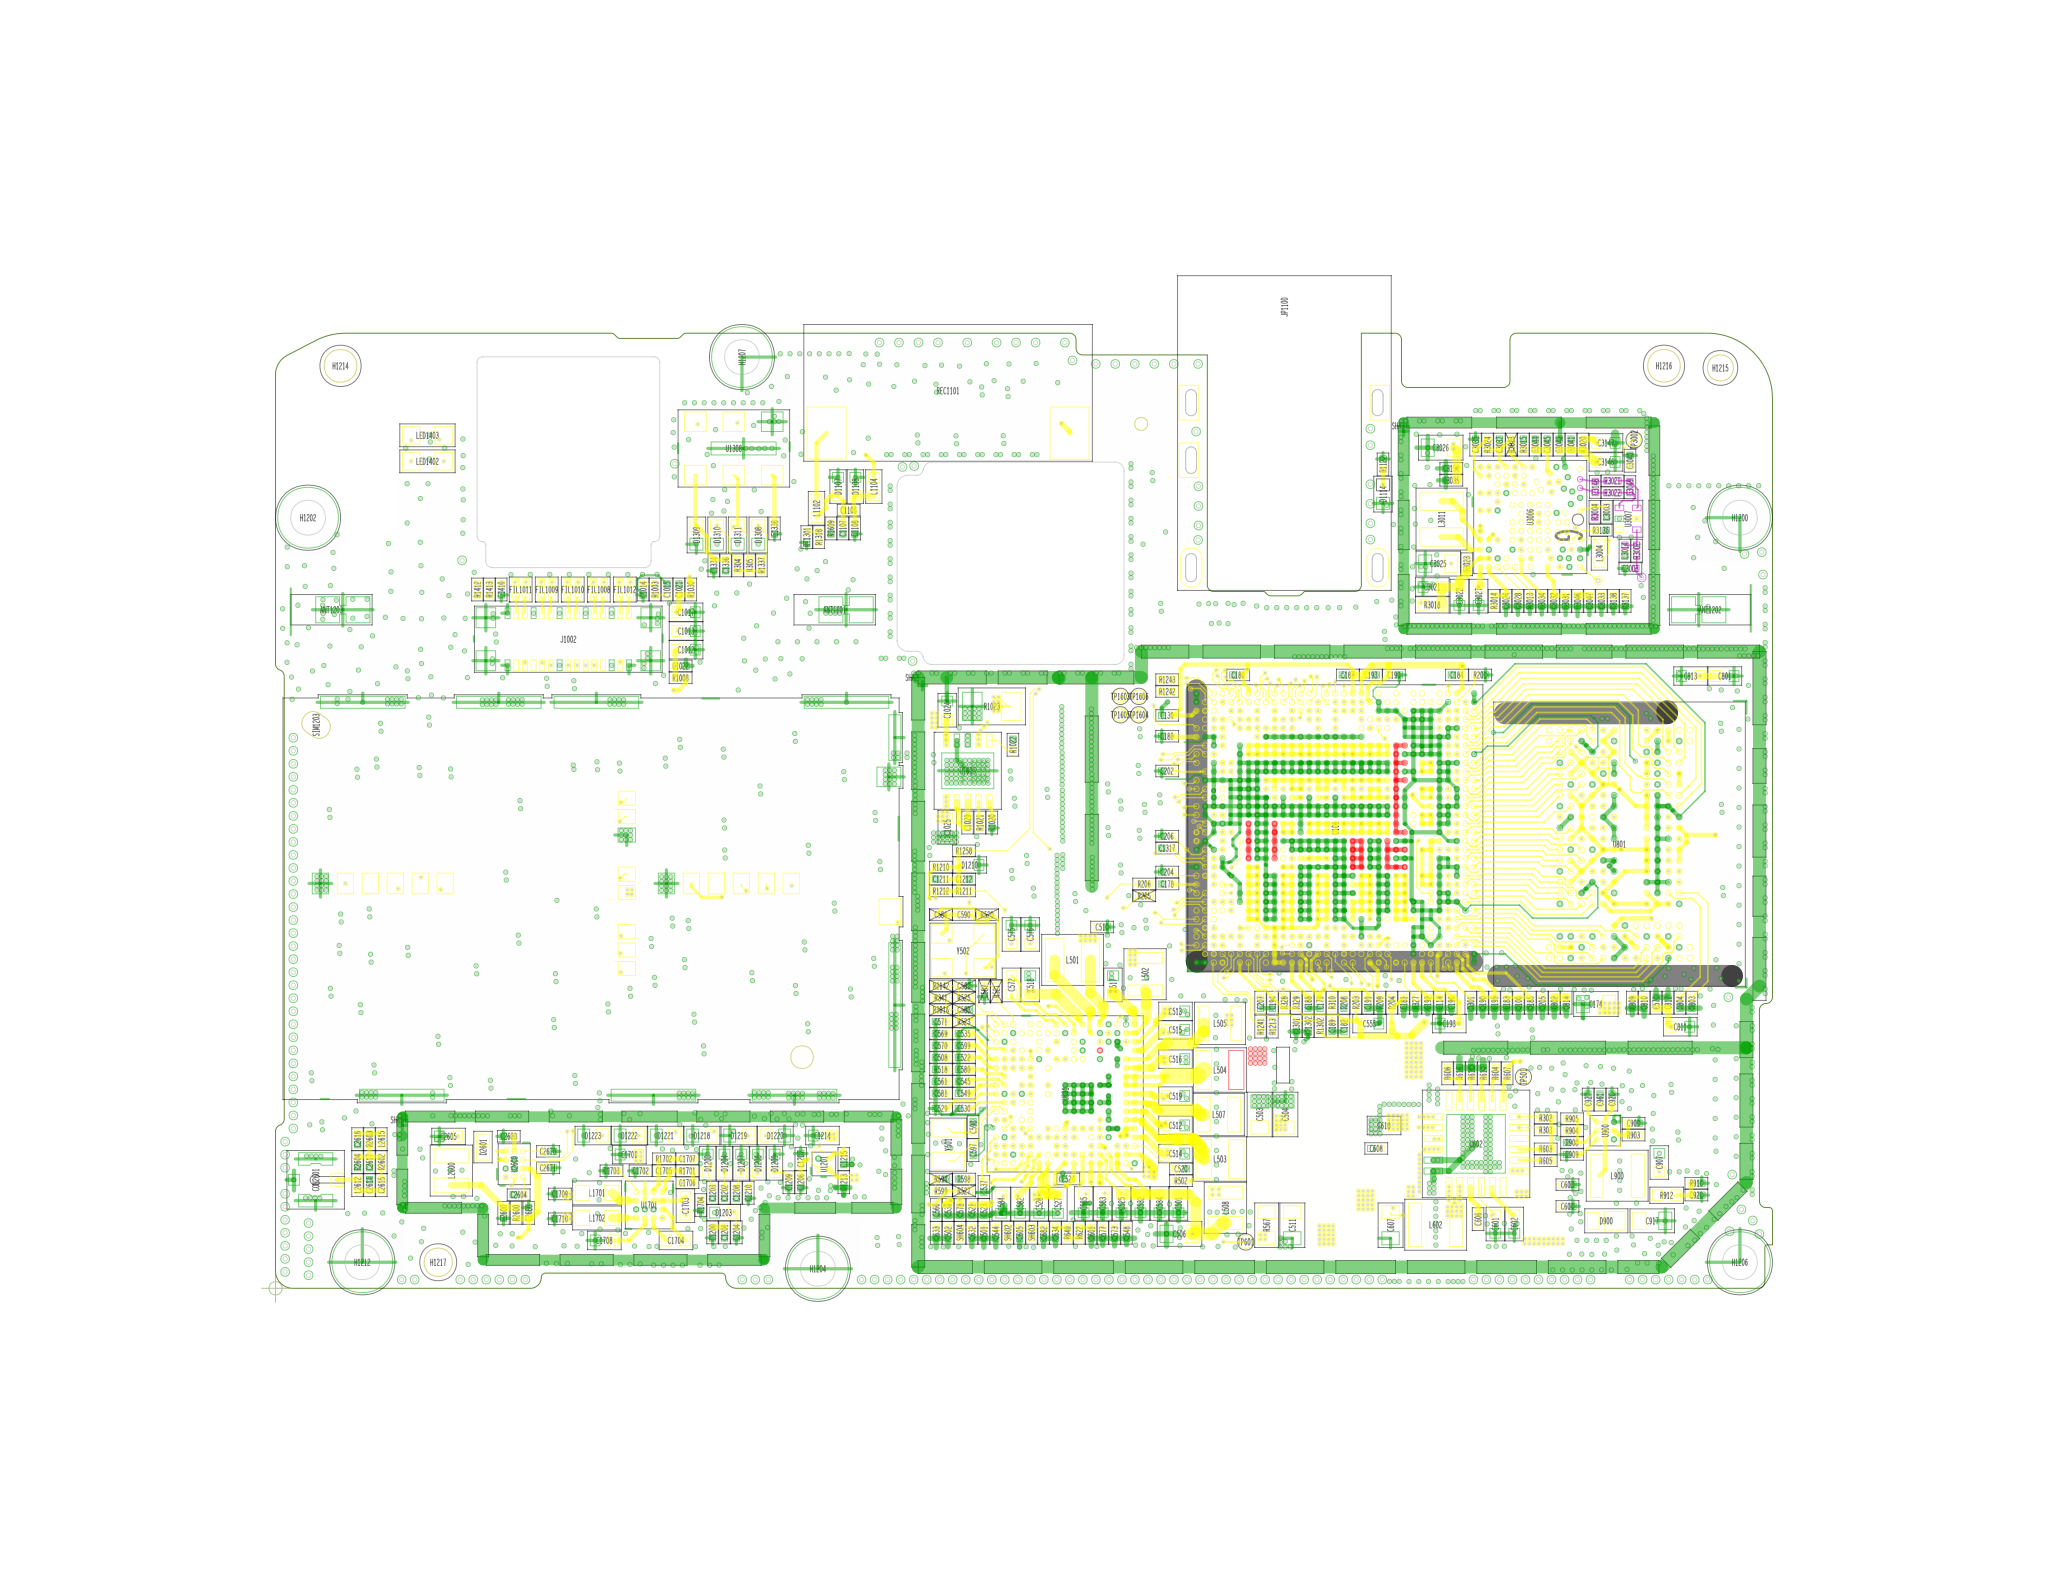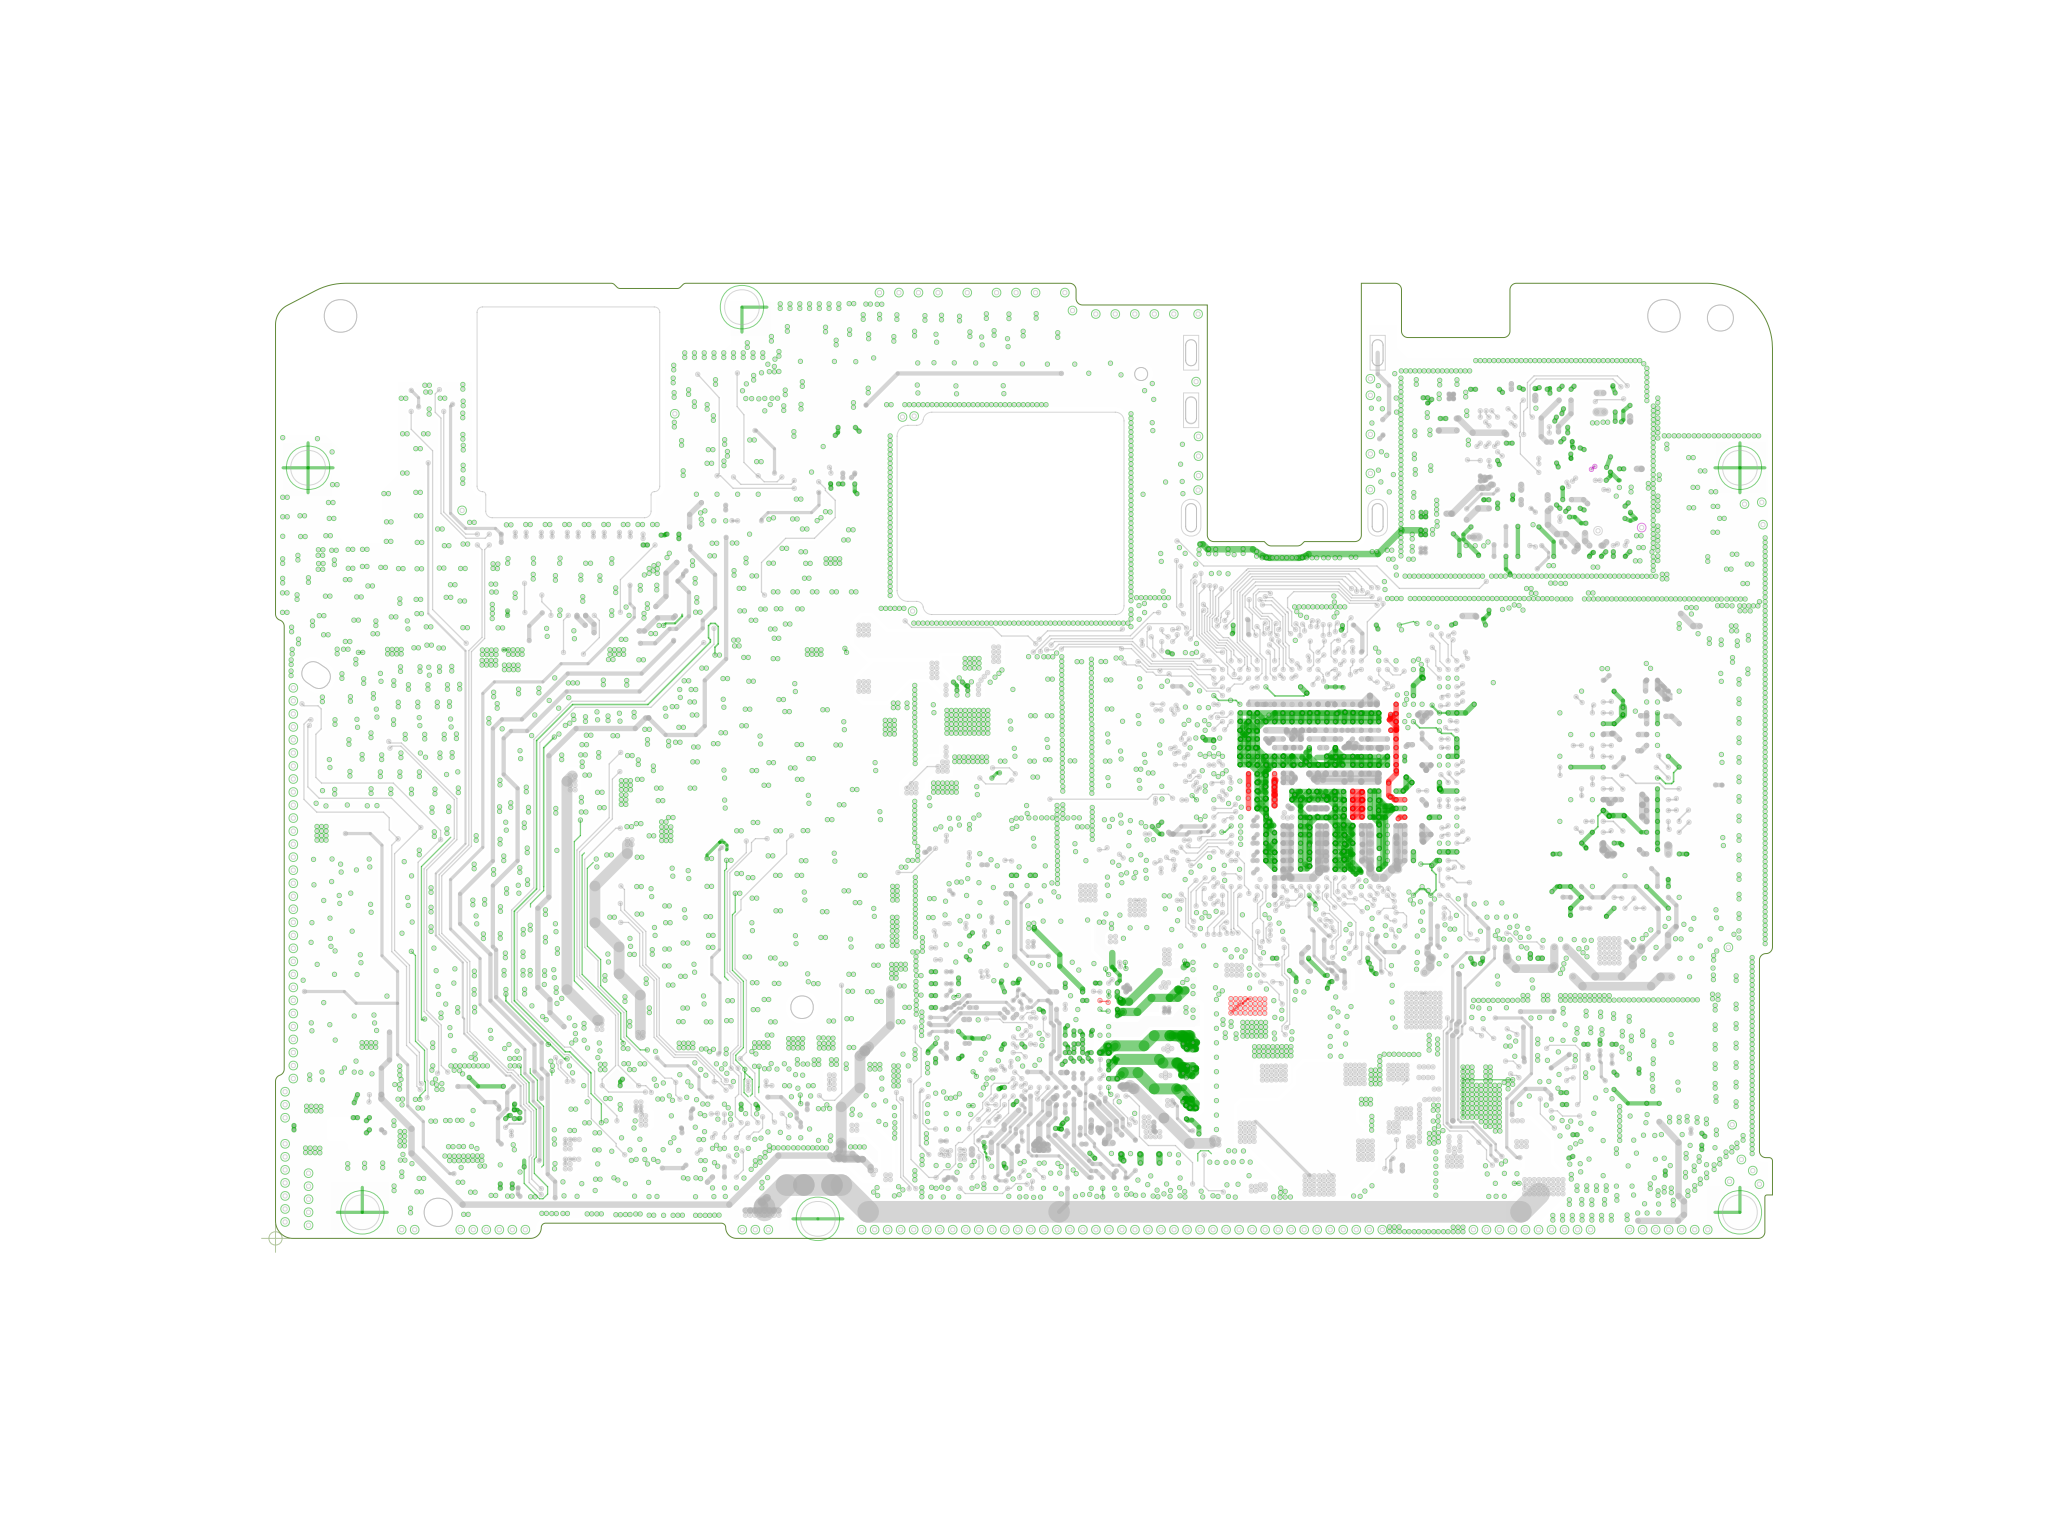Circuit board layout | Cadence Allegro
Layer stack:
# Cadence Allegro layer stack of  (unit mm; from the constraint file cross-section; dielectric type: 0 not recorded (Allegro does not mark core vs prepreg), 3 surface material)
index,name,kind,layer,copper_thickness_mm,dielectric_type,dielectric_thickness_mm,dielectric_material,dielectric_constant
0,Top Surface,other,,,,,,
1,TOP,copper,TOP,0.0305,,,,
2,Dielectric1,dielectric,,,0,0.2032,FR-4,4.5
3,L2,copper,L2,0.0305,,,,
4,Dielectric2,dielectric,,,0,0.2032,FR-4,4.5
5,L3,copper,L3,0.0305,,,,
6,Dielectric3,dielectric,,,0,0.2032,FR-4,4.5
7,L4,copper,L4,0.0305,,,,
8,Dielectric4,dielectric,,,0,0.2032,FR-4,4.5
9,L5,copper,L5,0.0305,,,,
10,Dielectric5,dielectric,,,0,0.2032,FR-4,4.5
11,L6,copper,L6,0.0305,,,,
12,Dielectric6,dielectric,,,0,0.2032,FR-4,4.5
13,L7,copper,L7,0.0305,,,,
14,Dielectric7,dielectric,,,0,0.2032,FR-4,4.5
15,L8,copper,L8,0.0305,,,,
16,Dielectric8,dielectric,,,0,0.2032,FR-4,4.5
17,L9,copper,L9,0.0305,,,,
18,Dielectric9,dielectric,,,0,0.2032,FR-4,4.5
19,BOTTOM,copper,BOTTOM,0.0305,,,,
20,Bottom Surface,other,,,,,,
# drill layer pairs: low layer,high layer
drill_pair,TOP,BOTTOM
Part placement, first 568 of 1093 lines:
REFDES,COMP_VALUE,SYM_NAME,SYM_X,SYM_Y,SYM_ROTATE,SYM_MIRROR
ANT1201,K3.1.21.0113,PIN_ANT_K3_1_21_0113,25.775,31.26,0.000,NO
ANT1202,K3.1.21.0113,PIN_ANT_K3_1_21_0113,66.125,31.26,180.000,NO
ANT1203,K3.1.21.0113,PIN_ANT_K3_1_21_0113,2.577,31.26,0.000,NO
ANT1204,818001102,PIN_ANT_818001102,34.63,7.82,270.000,YES
ANT1205,818001103,PIN_ANT_818001103,1.5,29.995,180.000,YES
ANT1206,818001103,PIN_ANT_818001103,67.3,29.895,180.000,YES
ANT1207,818001105,PIN_ANT_818001105,40.21,34.275,180.000,YES
ANT2600,818001475,PIN_ANT_818001475,2.1,39.695,270.000,YES
ANT2601,818001475,PIN_ANT_818001475,4.3,39.695,270.000,YES
ANT2605,818001475,PIN_ANT_818001475,6.37,41.745,90.000,YES
ANT3000,818001475,PIN_ANT_818001475,64.5,39.345,270.000,YES
ANT3001,818001475,PIN_ANT_818001475,60.375,42.12,180.000,YES
ANT3002,818001475,PIN_ANT_818001475,66.7,39.495,270.000,YES
C100,1UF,C0201,57.29,13.156,270.000,NO
C101,470nF,C0201,48.803,21.187,270.000,YES
C102,470nF,C0201,50.453,21.187,270.000,YES
C103,470nF,C0201,49.903,21.187,270.000,YES
C104,470nF,C0201,48.253,21.187,270.000,YES
C105,4.7uF,0402-BIG,52.301,16.886,90.000,YES
C106,470nF,C0201,50.453,23.307,270.000,YES
C107,470nF,C0201,49.903,23.307,270.000,YES
C109,10UF,0603-BIG,54.614,17.126,90.000,YES
C110,1UF,C0201,50.453,17.717,90.000,YES
C111,1UF,C0201,51.553,17.717,90.000,YES
C112,470nF,C0201,48.253,23.307,270.000,YES
C113,1UF,C0201,51.553,16.657,90.000,YES
C114,100NF,C0201,53.652,13.156,270.000,NO
C115,1UF,C0201,50.453,18.777,270.000,YES
C116,2.2UF,0402-BIG,52.301,20.042,270.000,YES
C117,1UF,C0201,51.553,18.777,270.000,YES
C118,1UF,C0201,51.553,20.127,270.000,YES
C119,1UF,C0201,52.103,22.247,90.000,YES
C123,1UF,C0201,46.055,19.075,90.000,YES
C124,1UF,C0201,45.356,21.22,270.000,YES
C125,1UF,C0201,52.1,24.367,270.000,YES
C126,22UF,0603-BIG,46.648,23.263,0.000,YES
C131,1UF,C0201,50.453,16.657,90.000,YES
C133,1UF,C0201,50.453,20.127,270.000,YES
C136,47UF,0603-BIG,48.88,14.25,90.000,YES
C138,47UF,0603-BIG,47.7,14.25,90.000,YES
C139,100NF,C0201,41.1,26.392,180.000,NO
C140,47UF,0603-BIG,46.53,14.25,90.000,YES
C141,4.7uF,0402-BIG,49.86,12.016,90.000,YES
C142,22UF,0603-BIG,46.648,25.433,0.000,YES
C143,4.7uF,0402-BIG,51.606,21.285,180.000,YES
C144,4.7uF,0402-BIG,51.606,25.325,180.000,YES
C145,4.7uF,0402-BIG,51.606,23.205,180.000,YES
C146,47UF,0603-BIG,53.41,17.126,90.000,YES
C147,470nF,C0201,48.803,23.307,270.000,YES
C148,2.2UF,0402-BIG,44.31,14.006,90.000,YES
C149,22UF,0603-BIG,46.648,21.233,0.000,YES
C150,1UF,C0201,48.253,16.657,270.000,YES
C151,1UF,C0201,48.803,16.657,270.000,YES
C152,1UF,C0201,48.253,17.717,90.000,YES
C153,1UF,C0201,48.253,18.777,270.000,YES
C154,1UF,C0201,47.703,16.657,270.000,YES
C155,47UF,0603-BIG,45.356,14.25,90.000,YES
C158,1UF,C0201,45.505,17.717,90.000,YES
C159,1UF,C0201,46.055,16.657,270.000,YES
C160,1UF,C0201,45.505,16.657,270.000,YES
C161,1UF,C0201,47.703,17.717,90.000,YES
C162,1UF,C0201,48.803,17.717,90.000,YES
C163,1UF,C0201,46.055,17.717,90.000,YES
C164,1UF,C0201,48.803,18.777,270.000,YES
C168,470nF,C0201,48.803,25.427,90.000,YES
C169,470nF,C0201,50.453,25.427,90.000,YES
C170,470nF,C0201,48.253,25.427,90.000,YES
C171,470nF,C0201,49.903,25.427,90.000,YES
C172,100NF,C0201,53.2,23.307,90.000,YES
C173,100NF,C0201,53.2,20.127,270.000,YES
C174,10UF,0603-BIG,60.86,13.096,180.000,NO
C175,4.7uF,0402-BIG,54.38,23.213,180.000,YES
C176,100NF,C0201,53.2,21.187,90.000,YES
C177,100NF,C0201,53.2,22.247,90.000,YES
C178,1UF,C0201,41.11,18.626,180.000,NO
C179,1UF,C0201,48.148,13.156,90.000,NO
C180,100NF,C0201,41.1,25.433,180.000,NO
C181,100NF,C0201,52.002,13.156,270.000,NO
C182,100NF,C0201,49.248,12.081,270.000,NO
C183,100NF,C0201,56.74,13.156,270.000,NO
C184,100NF,C0201,54.457,28.256,180.000,NO
C185,100NF,C0201,57.84,13.156,270.000,NO
C186,100NF,C0201,44.373,28.256,180.000,NO
C187,100NF,C0201,49.428,28.256,180.000,NO
C188,100NF,C0201,47.598,13.156,270.000,NO
C189,100NF,C0201,48.698,12.081,270.000,NO
C190,100NF,C0201,55.64,13.156,270.000,NO
C191,1UF,C0201,50.348,13.156,270.000,NO
C192,100NF,C0201,53.102,13.156,270.000,NO
C193,1UF,C0201,50.489,28.256,0.000,NO
C194,1UF,C0201,45.952,13.156,270.000,NO
C195,1UF,C0201,56.19,13.156,270.000,NO
C196,100NF,C0201,54.202,13.156,270.000,NO
C197,100NF,C0201,45.505,19.075,90.000,YES
C198,4.7uF,0402-BIG,54.102,12.195,180.000,NO
C199,100NF,C0201,51.551,28.256,0.000,NO
C201,1UF,C0201,53.2,24.367,270.000,YES
C202,100NF,C0201,41.1,23.832,180.000,NO
C204,1UF,C0201,41.1,19.178,180.000,NO
C205,100NF,C0201,58.39,13.156,270.000,NO
C206,100NF,C0201,41.1,20.828,0.000,NO
C207,100NF,C0201,45.402,13.156,90.000,NO
C501,10UF,0402-BIG,41.62,3.906,270.000,NO
C502,1UF,C0201,31,2.556,90.000,NO
C503,22UF,0603-BIG,45.363,8.007,90.000,NO
C504,22UF,0603-BIG,46.547,8.007,90.000,NO
C506,22UF,0603-BIG,41.67,2.506,180.000,NO
C508,1UF,C0201,30.674,10.635,0.000,NO
C510,1UF,C0201,38.097,16.643,180.000,NO
C511,22UF,0603-BIG,46.867,2.906,270.000,NO
C512,2.2UF,0402-BIG,41.484,7.506,0.000,NO
C513,2.2UF,0402-BIG,41.484,12.756,0.000,NO
C514,2.2UF,0402-BIG,41.484,6.206,0.000,NO
C515,2.2UF,0402-BIG,41.484,11.906,0.000,NO
C516,2.2UF,0402-BIG,41.484,10.556,0.000,NO
C517,4.7uF,0402-BIG,38.602,13.976,90.000,NO
C518,2.2UF,0402-BIG,34.788,13.976,90.000,NO
C519,2.2UF,0402-BIG,41.484,8.856,0.000,NO
C520,1UF,C0201,41.736,5.506,180.000,NO
C521,1UF,C0201,32.1,3.606,90.000,NO
C522,1UF,C0201,31.734,10.635,0.000,NO
C523,1UF,C0201,32.65,3.606,90.000,NO
C524,1UF,C0201,36.539,5.036,0.000,NO
C525,4.7uF,0402-BIG,38.995,3.906,270.000,NO
C527,2.2UF,0402-BIG,36.064,3.879,90.000,NO
C528,2.2UF,0402-BIG,35.201,3.879,90.000,NO
C529,1UF,C0201,30.674,8.285,0.000,NO
C530,1UF,C0201,31.734,8.285,0.000,NO
C532,4.7uF,0402-BIG,39.87,3.906,270.000,NO
C533,100NF,C0201,31,3.606,270.000,NO
C534,4.7uF,0402-BIG,40.745,3.906,270.000,NO
C535,1UF,C0201,31.734,11.735,0.000,NO
C537,100NF,C0201,32.65,4.666,90.000,NO
C544,1UF,C0201,33.2,2.556,90.000,NO
C545,1UF,C0201,31.734,9.535,0.000,NO
C548,1UF,C0201,39.225,2.556,90.000,NO
C549,1UF,C0201,31.734,8.985,0.000,NO
C555,4.7uF,0402-BIG,50.429,12.194,0.000,NO
C561,1UF,C0201,30.674,9.535,0.000,NO
C566,100NF,C0201,30.45,3.606,90.000,NO
C569,1UF,C0201,30.674,11.735,180.000,NO
C570,1UF,C0201,30.674,11.185,180.000,NO
C571,1UF,C0201,30.674,12.285,180.000,NO
C572,4.7uF,0402-BIG,33.922,13.976,270.000,NO
C573,1UF,C0201,38.675,2.556,270.000,NO
C575,2.2UF,0402-BIG,33.922,16.3,90.000,NO
C576,4.7uF,0402-BIG,34.788,16.3,270.000,NO
C577,1UF,C0201,38.13,2.556,90.000,NO
C578,1UF,C0201,31.55,3.606,90.000,NO
C579,1UF,C0201,63.635,13.156,270.000,NO
C580,1UF,C0201,31.734,10.085,0.000,NO
C581,1UF,C0201,30.674,8.985,0.000,NO
C582,4.7uF,0402-BIG,34.321,3.879,270.000,NO
C583,4.7uF,0402-BIG,38.125,3.906,270.000,NO
C584,2.2UF,0402-BIG,33.45,3.881,270.000,NO
C585,4.7uF,0402-BIG,37.25,3.906,270.000,NO
C586,NM,0201_NM,30.674,17.215,0.000,NO
C587,NM,0201_NM,32.68,13.682,270.000,NO
C588,NM,0201_NM,31.734,12.835,0.000,NO
C589,NM,0201_NM,31.734,13.935,0.000,NO
C590,0R,R0201,31.73,17.215,180.000,NO
C597,22PF,C0201,32.155,6.367,270.000,NO
C598,22PF,C0201,32.155,7.427,90.000,NO
C599,1UF,C0201,31.734,11.185,180.000,NO
C601,4.7uF,0402-BIG,56.226,2.96,270.000,NO
C602,10UF,0402-BIG,57.101,2.96,270.000,NO
C603,1UF,C0201,59.549,4.775,0.000,NO
C604,22nF,C0201,59.549,3.775,0.000,NO
C605,1UF,C0201,34.3,2.556,90.000,NO
C606,47nF,C0201,55.429,3.187,90.000,NO
C607,22UF,0603-BIG,51.398,2.906,270.000,NO
C608,1UF,C0201,50.737,6.442,180.000,NO
C610,10UF,0402-BIG,51.097,7.5,180.000,NO
C612,100NF,C0201,57.702,4.837,180.000,YES
C632,1UF,C0201,32.1,2.556,270.000,NO
C633,1UF,C0201,30.45,2.556,270.000,NO
C634,1UF,C0201,35.95,2.556,270.000,NO
C682,1UF,C0201,35.4,2.556,90.000,NO
C736,10UF,0402-BIG,55.26,11.626,180.000,YES
C737,10UF,0402-BIG,55.26,15.636,180.000,YES
C742,1UF,C0201,57.41,14.366,180.000,YES
C745,1UF,C0201,57.41,13.386,180.000,YES
C801,2.2UF,0402-BIG,66.804,28.207,0.000,NO
C802,100NF,C0201,58.943,13.156,270.000,NO
C803,10UF,0402-BIG,60.599,24.039,0.000,YES
C804,10UF,0402-BIG,60.599,24.949,0.000,YES
C805,100NF,C0201,60.837,20.244,0.000,YES
C806,100NF,C0201,60.837,19.694,0.000,YES
C807,100NF,C0201,60.837,23.247,0.000,YES
C808,100NF,C0201,60.837,22.697,0.000,YES
C809,100NF,C0201,62.535,13.156,270.000,NO
C810,1UF,C0201,63.085,13.156,270.000,NO
C811,4.7uF,0402-BIG,64.753,12.049,0.000,NO
C812,220NF,C0201,64.185,13.156,90.000,NO
C813,2.2UF,0402-BIG,65.225,28.207,180.000,NO
C814,100NF,C0201,59.493,13.156,270.000,NO
C815,1UF,C0201,60.837,21.894,0.000,YES
C816,100NF,C0201,60.837,21.344,0.000,YES
C907,10UF,0402-BIG,63.784,5.794,90.000,NO
C908,100NF,C0201,55.785,8.261,90.000,YES
C909,1UF,C0201,62.597,7.607,0.000,NO
C916,4.7uF,0402-BIG,59.493,11.798,270.000,YES
C917,1UF,C0603,63.459,3.109,0.000,NO
C919,2.2uF,0603-BIG,59.72,9.946,90.000,YES
C920,4.7uF,0402-BIG,59.497,13.414,90.000,YES
C921,10UF,0402-BIG,57.16,8.256,180.000,YES
C922,4.7uF,0402-BIG,60.59,8.106,0.000,YES
C926,33PF,C0201,61.601,8.692,90.000,NO
C927,33PF,C0201,60.501,8.692,90.000,NO
C928,33PF,C0201,65.492,4.293,0.000,NO
C929,1UF,C0201,60.837,11.694,180.000,YES
C930,56pF,C0201,60.837,11.144,180.000,YES
C931,56pF,C0201,60.837,10.594,180.000,YES
C932,1UF,C0201,52.63,31.906,180.000,YES
C961,33PF,C0201,61.051,8.692,90.000,NO
C1000,1UF,C0201,22.886,31.113,270.000,YES
C1004,2.2UF,0402-BIG,22.357,32.144,0.000,YES
C1005,4.7uF,0402-BIG,22.357,33.008,0.000,YES
C1006,100NF,C0201,22.597,33.753,0.000,YES
C1007,4.7uF,0402-BIG,22.357,35.1,0.000,YES
C1008,100NF,C0201,22.597,34.305,0.000,YES
C1010,22PF,C0201,22.597,35.858,0.000,YES
C1011,22PF,C0201,22.597,36.973,180.000,YES
C1012,4.7uF,0402-BIG,18.923,29.419,0.000,NO
C1013,2.2UF,0402-BIG,18.924,30.278,0.000,NO
C1014,22PF,C0201,16.943,32.193,270.000,NO
C1015,22PF,C0201,18.043,32.193,90.000,NO
C1017,4.7uF,0402-BIG,18.923,31.144,0.000,NO
C1021,100NF,C0201,18.593,32.193,90.000,NO
C1022,100NF,C0201,18.673,28.673,0.000,NO
C1024,4.7uF,0402-BIG,30.961,26.629,90.000,NO
C1025,10UF,0402-BIG,30.961,21.235,270.000,NO
C1026,100NF,C0201,40.074,37.801,90.000,YES
C1029,1UF,C0201,31.898,21.455,90.000,NO
C1101,1nF,C0201,52.63,30.806,180.000,YES
C1102,1nF,C0201,40.89,36.956,180.000,YES
C1104,33PF,C0201,44.514,26.252,0.000,YES
C1105,33PF,C0201,52.81,28.506,180.000,YES
C1106,100PF,C0201,26.419,35.848,180.000,NO
C1107,33PF,C0201,26.15,35.006,270.000,NO
C1108,33PF,C0201,26.7,35.006,270.000,NO
C1109,33PF,C0201,31.3,42.056,0.000,YES
C1110,1UF,C0201,31.3,42.606,0.000,YES
C1111,82PF,C0201,48.01,28.506,180.000,YES
C1112,100NF,C0201,44.514,25.702,0.000,YES
C1114,33PF,C0201,28.598,42.056,0.000,YES
C1115,100NF,C0201,30.2,42.606,0.000,YES
C1116,33PF,C0201,41.286,26.249,180.000,YES
C1120,1nF,C0201,44.55,28.506,180.000,YES
C1121,33PF,C0201,29.931,40.624,0.000,YES
C1122,33PF,C0201,40.226,26.802,0.000,YES
C1123,1UF,C0201,40.885,31.41,0.000,YES
C1124,1nF,C0201,46.95,28.506,180.000,YES
C1125,1nF,C0201,51.7,28.506,0.000,YES
C1126,33PF,C0201,43.49,28.506,0.000,YES
C1200,22PF,C0201,20.142,2.576,270.000,NO
C1201,1UF,C0201,20.692,2.576,270.000,NO
C1202,22PF,C0201,20.692,4.396,270.000,NO
C1203,22PF,C0201,20.142,4.396,270.000,NO
C1204,22PF,C0201,21.242,2.576,270.000,NO
C1205,100NF,C0201,59.277,18.594,180.000,YES
C1206,22PF,C0201,24.208,4.886,270.000,NO
C1207,1UF,C0201,24.208,5.956,90.000,NO
C1208,22PF,C0201,21.242,4.396,270.000,NO
C1209,22PF,C0201,23.658,4.886,270.000,NO
C1210,22PF,C0201,21.792,4.396,270.000,NO
C1211,1UF,C0201,30.674,18.855,180.000,NO
C1212,22PF,C0201,31.734,18.855,0.000,NO
C1213,1UF,C0201,26.192,4.886,270.000,NO
C1214,4.7uF,0402-BIG,25.211,7.036,180.000,NO
C1215,100NF,C0201,26.192,5.956,270.000,NO
C1300,100NF,C0201,59.777,23.247,0.000,YES
C1301,100NF,C0201,47.048,12.081,90.000,NO
C1314,100NF,C0201,54.627,28.979,180.000,YES
C1315,100NF,C0201,56.227,29.056,180.000,YES
C1316,1UF,C0201,56.227,28.506,180.000,YES
C1317,100NF,C0201,41.1,20.278,0.000,NO
C1325,1UF,C0201,51.892,8.261,90.000,YES
C1327,1UF,C0201,54.513,8.261,90.000,YES
C1328,1UF,C0201,53.681,8.261,90.000,YES
C1332,100NF,C0201,60.837,19.144,180.000,YES
C1334,1UF,C0201,20.2,33.306,270.000,NO
C1336,100NF,C0201,20.75,33.306,90.000,NO
C1338,1UF,C0201,23,35.006,270.000,NO
C1410,1UF,C0201,10.404,32.193,90.000,NO
C1429,100PF,C0201,17.127,1.612,270.000,YES
C1430,1UF,C0201,16.027,1.612,90.000,YES
C1502,33PF,C0201,18.227,1.612,90.000,YES
C1504,100NF,C0201,15.477,1.612,90.000,YES
C1507,10PF,C0201,15.06,5.935,270.000,YES
C1508,10PF,C0201,14.506,5.935,270.000,YES
C1512,1UF,C0201,18.777,1.612,90.000,YES
C1513,100NF,C0201,17.677,1.612,90.000,YES
C1514,100NF,C0201,52.994,8.261,90.000,YES
C1515,100NF,C0201,51.357,8.261,90.000,YES
C1516,100NF,C0201,14.927,1.612,90.000,YES
C1605,100NF,C0201,33.412,19.175,90.000,YES
C1606,100NF,C0201,31.762,19.175,90.000,YES
C1607,100NF,C0201,32.312,19.175,90.000,YES
C1608,2.2UF,0402-BIG,30.841,23.803,90.000,YES
C1609,2.2UF,0402-BIG,35.027,18.923,270.000,YES
C1610,1UF,C0201,30.924,24.889,180.000,YES
C1611,4.7uF,0402-BIG,34.167,18.923,270.000,YES
C1612,1UF,C0201,30.924,21.639,0.000,YES
C1613,100NF,C0201,32.862,19.175,90.000,YES
C1614,1UF,C0201,38.106,25.699,0.000,YES
C1616,1UF,C0201,38.106,26.249,0.000,YES
C1617,2.2UF,0402-BIG,36.257,26.338,90.000,YES
C1618,4.7uF,0402-BIG,34.537,26.338,90.000,YES
C1619,4.7uF,0402-BIG,33.677,26.338,90.000,YES
C1620,1UF,C0201,39.166,25.699,0.000,YES
C1621,1UF,C0201,40.226,26.249,0.000,YES
C1622,1UF,C0201,15.61,5.935,270.000,YES
C1623,2.2UF,0402-BIG,35.397,26.338,90.000,YES
C1624,1UF,C0201,13.947,5.935,270.000,YES
C1625,1UF,C0201,39.166,26.802,0.000,YES
C1626,470nF,C0201,38.106,26.802,180.000,YES
C1627,1UF,C0201,39.166,26.249,0.000,YES
C1628,2.2UF,0402-BIG,39.692,20.965,180.000,YES
C1629,4.7uF,0402-BIG,32.817,26.338,90.000,YES
C1630,2.2UF,0402-BIG,39.692,23.566,180.000,YES
C1631,2.2UF,0402-BIG,39.692,22.698,180.000,YES
C1632,2.2UF,0402-BIG,39.692,21.831,180.000,YES
C1633,4.7uF,0402-BIG,31.957,26.338,90.000,YES
C1634,4.7uF,0402-BIG,39.692,24.434,0.000,YES
C1636,1UF,C0201,38.516,22.441,90.000,YES
C1638,4.7uF,0402-BIG,37.117,26.338,90.000,YES
C1640,1UF,C0201,35.797,18.675,90.000,YES
C1641,1UF,C0201,38.584,18.51,180.000,YES
C1701,4.7uF,0402-BIG,16.311,6.161,180.000,NO
C1702,100NF,C0201,16.827,5.414,180.000,NO
C1703,2.2UF,0402-BIG,18.893,3.804,90.000,NO
C1704,2.2UF,0402-BIG,18.458,2.206,0.000,NO
C1705,220PF,C0201,17.905,5.414,180.000,NO
C1706,100NF,C0201,18.985,4.864,0.000,NO
C1707,100NF,C0201,18.985,5.969,180.000,NO
C1708,4.7uF,0402-BIG,15.159,2.205,180.000,NO
C1709,1nF,C0201,13.11,4.346,180.000,NO
C1710,1nF,C0201,13.11,3.206,180.000,NO
C2100,100NF,C0201,17.717,14.497,180.000,YES
C2101,100NF,C0201,18.565,10.838,90.000,YES
C2102,10nF,C0201,26.533,10.219,180.000,YES
C2103,100NF,C0201,17.717,11.097,180.000,YES
C2104,0R,R0201,22.916,10.838,270.000,YES
C2106,1nF,C0201,24.135,8.228,90.000,YES
C2108,100NF,C0201,25.473,10.769,0.000,YES
C2109,1nF,C0201,25.473,12.419,180.000,YES
C2110,100NF,C0201,26.533,11.869,0.000,YES
C2111,100NF,C0201,19.115,10.838,90.000,YES
C2112,100NF,C0201,26.533,9.669,0.000,YES
C2114,100NF,C0201,17.717,10.547,180.000,YES
C2200,1.2PF,C0201,4.354,20.049,0.000,YES
C2201,1.2PF,C0201,4.354,21.149,180.000,YES
C2202,8.2PF,C0201,4.354,19.499,0.000,YES
C2205,33PF,C0201,17.717,12.497,180.000,YES
C2206,1PF,C0201,16.9,12.747,270.000,YES
C2207,1PF,C0201,4.354,25.549,0.000,YES
C2210,1nF,C0201,4.354,22.799,0.000,YES
C2211,33PF,C0201,4.354,27.749,0.000,YES
C2212,100NF,C0201,4.354,23.899,0.000,YES
C2213,10PF,C0201,4.354,23.349,0.000,YES
C2214,1UF,C0201,9.674,23.349,180.000,YES
C2215,100PF,C0201,9.674,23.899,180.000,YES
C2216,1UF,C0201,9.674,22.249,180.000,YES
C2217,100PF,C0201,9.674,22.799,180.000,YES
C2218,15PF,C0201,6.474,19.499,0.000,YES
C2220,3.3PF,C0201,4.354,27.199,180.000,YES
C2221,NM,0201_NM,6.474,18.949,0.000,YES
C2222,3.3PF,C0201,4.354,26.099,0.000,YES
C2223,1UF,C0201,4.354,18.399,0.000,YES
C2224,NM,0402_NM,14.094,8.018,180.000,YES
C2225,4.7uF,0402-BIG,11.069,23.189,180.000,YES
C2226,NM,0201_NM,5.414,18.949,180.000,YES
C2227,15PF,C0201,5.414,19.499,180.000,YES
C2228,1PF,C0201,4.354,21.699,0.000,YES
C2229,1PF,C0201,16.9,13.847,270.000,YES
C2230,33PF,C0201,17.717,13.597,180.000,YES
C2300,15PF,C0201,9.674,19.499,180.000,YES
C2301,33PF,C0201,9.674,26.099,180.000,YES
C2302,33PF,C0201,4.354,28.849,0.000,YES
C2303,33PF,C0201,9.674,27.199,180.000,YES
C2304,33PF,C0201,5.414,28.849,0.000,YES
C2305,15PF,C0201,7.534,19.499,180.000,YES
C2306,33PF,C0201,6.474,28.849,0.000,YES
C2307,33PF,C0201,9.674,28.849,180.000,YES
C2308,33PF,C0201,7.534,28.849,180.000,YES
C2309,33PF,C0201,9.674,24.449,180.000,YES
C2310,15PF,C0201,11.31,19.212,90.000,YES
C2311,33PF,C0201,9.674,21.149,180.000,YES
C2312,33PF,C0201,17.717,21.309,0.000,YES
C2313,33PF,C0201,18.569,21.04,90.000,YES
C2314,33PF,C0201,10.824,25.549,0.000,YES
C2315,33PF,C0201,14.894,27.749,0.000,YES
C2316,33PF,C0201,15.194,23.187,270.000,YES
C2317,33PF,C0201,10.824,26.649,0.000,YES
C2318,33PF,C0201,8.594,28.849,180.000,YES
C2319,33PF,C0201,17.717,18.547,0.000,YES
C2330,33PF,C0201,21.319,19.98,270.000,YES
C2400,NM,0201_NM,13.834,10.683,180.000,YES
C2401,10PF,C0201,13.834,10.133,180.000,YES
C2402,1nF,C0201,13.834,9.583,180.000,YES
C2403,22uF,0402-BIG,14.094,8.868,180.000,YES
C2404,33PF,C0201,14.894,13.983,0.000,YES
C2405,10nF,C0201,13.834,11.233,180.000,YES
C2410,18PF,C0201,13.834,12.333,0.000,YES
C2411,NM,0201_NM,13.834,11.783,0.000,YES
C2500,1nF,C0201,20.855,24.629,180.000,YES
C2502,1nF,C0201,20.855,25.729,180.000,YES
C2504,1nF,C0201,20.855,24.079,180.000,YES
C2513,1UF,C0201,20.855,26.932,180.000,YES
C2555,1nF,C0201,20.855,25.179,180.000,YES
C2600,1UF,C0201,10.511,3.471,270.000,NO
C2603,100NF,C0201,10.754,7.003,0.000,NO
C2604,220NF,C0201,11.207,4.312,180.000,NO
C2605,47nF,C0402,7.976,6.997,180.000,NO
C2607,39pF,C0201,7.115,36.253,90.000,YES
C2610,5.1nH,L0201,5.905,36.268,90.000,YES
C2611,NM,0201_NM,6.725,35.418,180.000,YES
C2614,10PF,C0201,4.329,4.752,90.000,NO
C2615,33PF,C0201,4.879,4.752,90.000,NO
C2616,100PF,C0201,3.779,6.872,270.000,NO
C2617,100PF,C0201,4.329,5.812,270.000,NO
C2670,22PF,C0201,12.559,6.308,180.000,NO
C2671,22PF,C0201,12.559,5.551,0.000,NO
C2680,1UF,C0201,11.67,3.471,90.000,NO
C3003,3nH,L0201,62.45,33.161,180.000,NO
C3004,10NH,L0201,62.5,40.214,180.000,YES
C3005,NM,0201_NM,60.34,40.214,0.000,YES
C3014,1UF,C0201,60.031,32.756,0.000,YES
C3015,330PF,C0201,58.806,30.206,0.000,YES
C3016,18PF,C0201,60.031,35.806,0.000,YES
C3017,18PF,C0201,58.806,33.856,0.000,YES
C3020,1UF,C0201,61.969,32.206,180.000,YES
C3021,4.7uF,0402-BIG,53.32,32.311,0.000,NO
C3022,4.7uF,0402-BIG,54.57,31.886,90.000,NO
C3023,100NF,C0201,54.905,33.356,90.000,NO
C3024,1UF,C0201,56.715,31.666,270.000,NO
C3025,10UF,0603-BIG,53.595,33.386,180.000,NO
C3026,10UF,0603-BIG,53.71,38.726,180.000,NO
C3027,4.7uF,0402-BIG,55.455,31.886,90.000,NO
C3028,1UF,C0201,57.265,31.666,270.000,NO
C3029,1PF,C0201,60.031,31.656,180.000,YES
C3030,NM,0201_NM,60.031,31.106,180.000,YES
C3031,2.2uF,C0201,59.465,31.666,270.000,NO
C3032,10PF,C0201,58.915,31.666,270.000,NO
C3033,100NF,C0201,61.115,31.666,270.000,NO
C3034,100NF,C0201,58.365,31.666,270.000,NO
C3035,1UF,C0201,54.195,37.221,0.000,NO
C3037,100NF,C0201,56.415,38.866,90.000,NO
C3038,100NF,C0201,55.315,38.866,90.000,NO
C3040,10PF,C0201,62.435,38.123,90.000,NO
C3041,10PF,C0201,59.715,38.866,90.000,NO
C3042,5.6PF,C0201,59.165,38.866,270.000,NO
C3043,1nF,C0201,60.031,30.206,0.000,YES
C3044,10nF,C0201,58.065,38.866,90.000,NO
C3045,1UF,C0201,58.615,38.866,90.000,NO
C3046,100PF,C0201,60.015,31.666,270.000,NO
C3047,1UF,C0201,60.565,31.666,270.000,NO
C3049,2.2PF,C0201,62.43,36.911,270.000,NO
C3146,4.7uF,0402-BIG,61.325,38.071,180.000,NO
C3147,4.7uF,0402-BIG,61.325,38.946,180.000,NO
C3148,2.0pF,C0201,60.827,36.916,270.000,NO
C3149,100NF,C0201,63.769,32.206,180.000,YES
C3150,1UF,C0201,54.195,37.771,0.000,NO
C3190,1UF,C0201,12.774,21.149,0.000,YES
C3191,4.7uF,0402-BIG,19.802,9.42,270.000,YES
CON2400,818000291,RF_818000291,5.588,5.275,90.000,YES
CON2500,818000291,RF_818000291,6.481,33.813,270.000,YES
CON2601,818000500,RF_818000500,1.851,4.998,90.000,NO
CON3000,818000291,RF_818000291,60.76,38.606,270.000,YES
D601,VESD5451N-2/TR,DFN1006-2,53.937,0.841,180.000,YES
D602,VESD5451N-2/TR,DFN1006-2,52.268,0.84,0.000,YES
D612,VESD5621W04-2_TR,SOD-323F,53.56,5.81,0.000,YES
D624,VESD5451N-2/TR,DFN1006-2,55.656,5.409,90.000,YES
D900,WSB5523D,FBP1608-WSB5524D,61.341,3.109,180.000,NO
D902,VESD5451N-2/TR,DFN1006-2,56.6,33.036,270.000,YES
D903,VESD5451N-2/TR,DFN1006-2,54.05,33.036,270.000,YES
D904,VESD5451N-2/TR,DFN1006-2,53.2,33.036,270.000,YES
D905,VESD5451N-2/TR,DFN1006-2,55.75,33.036,270.000,YES
D906,VESD5451N-2/TR,DFN1006-2,54.9,33.036,270.000,YES
D907,VESD5451N-2/TR,DFN1006-2,60.883,12.844,90.000,YES
D1001,VESD5451N-2/TR,DFN1006-2,23.1,25.286,270.000,YES
D1101,VESD5311N-2/TR,DFN1006-2,48.52,29.6,270.000,YES
D1104,VESD5451N-2/TR,DFN1006-2,45.886,29.6,90.000,YES
D1105,VESD5451N-2/TR,DFN1006-2,51.824,29.6,90.000,YES
D1106,VESD5451N-2/TR,DFN1006-2,46.846,29.6,90.000,YES
D1107,AVLC18S02015,R0402_H0P7,25.928,36.934,90.000,NO
D1108,AVLC18S02015,R0402_H0P7,26.728,36.934,90.000,NO
D1109,VESD5451N-2/TR,DFN1006-2,43.44,29.6,270.000,YES
D1110,AVLC18S02015,R0402_H0P7,31.255,41.145,0.000,YES
D1111,AVLC18S02015,R0402_H0P7,29.931,41.924,180.000,YES
D1114,VESD5451N-2/TR,DFN1006-2,51.048,36.587,90.000,NO
D1115,AVLC18S02015,R0402_H0P7,28.882,42.723,180.000,YES
D1116,AVLC18S02015,R0402_H0P7,31.255,40.375,0.000,YES
D1200,AVLC18S02015,R0402_H0P7,19.922,5.756,90.000,NO
D1201,AVLC18S02015,R0402_H0P7,60.592,18.483,180.000,YES
D1202,AVLC18S02015,R0402_H0P7,60.592,17.723,180.000,YES
D1203,AVLC18S02015,R0402_H0P7,20.659,3.487,180.000,NO
D1204,AVLC18S02015,R0402_H0P7,20.692,5.756,90.000,NO
D1206,AVLC18S02015,R0402_H0P7,60.592,16.963,180.000,YES
D1207,AVLC18S02015,R0402_H0P7,21.462,5.756,90.000,NO
D1208,AVLC18S02015,R0402_H0P7,22.232,5.756,90.000,NO
D1209,AVLC18S02015,R0402_H0P7,23.002,5.756,90.000,NO
D1210,AVLC18S02015,R0402_H0P7,31.999,19.502,0.000,NO
D1218,VESD5311N-2/TR,DFN1006-2,19.656,7.036,0.000,NO
D1219,VESD5311N-2/TR,DFN1006-2,21.361,7.036,0.000,NO
D1220,VESD5311N-2/TR,DFN1006-2,23.039,7.036,180.000,NO
D1221,VESD5311N-2/TR,DFN1006-2,17.981,7.036,0.000,NO
D1222,VESD5311N-2/TR,DFN1006-2,16.311,7.036,0.000,NO
D1223,VESD5311N-2/TR,DFN1006-2,14.631,7.036,0.000,NO
D1308,VESD5451N-2/TR,DFN1006-2,22.25,34.706,90.000,NO
D1309,VESD5451N-2/TR,DFN1006-2,19.4,34.706,90.000,NO
D1310,VESD5451N-2/TR,DFN1006-2,20.35,34.706,90.000,NO
D1311,VESD5451N-2/TR,DFN1006-2,21.3,34.706,90.000,NO
D1502,VESD5311N-2/TR,DFN1006-2,18.382,5.997,180.000,YES
D1503,VESD5311N-2/TR,DFN1006-2,20.052,5.997,0.000,YES
D1509,VESD5451N-2/TR,DFN1006-2,16.717,5.997,180.000,YES
D1510,VESD5311N-2/TR,DFN1006-2,43.094,1.421,90.000,YES
D1511,VESD5311N-2/TR,DFN1006-2,43.094,4.181,270.000,YES
D1512,VESD5311N-2/TR,DFN1006-2,49.994,4.181,270.000,YES
D1513,VESD5311N-2/TR,DFN1006-2,49.994,1.421,90.000,YES
D1514,VESD5451N-2/TR,DFN1006-2,45.232,4.324,180.000,YES
D1515,VESD5451N-2/TR,DFN1006-2,46.914,4.324,0.000,YES
D1519,VESD5451N-2/TR,DFN1006-2,48.596,4.324,180.000,YES
D1520,AVLC18S02015,R0402_H0P7,60.592,16.193,180.000,YES
D2601,NSR05F40NXT5G,DSN2,9.563,6.506,270.000,NO
FIL905,EXC14CE900U,EXC14CE900U,66.851,6.562,270.000,YES
FIL906,EXC14CE900U,EXC14CE900U,66.851,8.962,270.000,YES
FIL907,EXC14CE900U,EXC14CE900U,66.851,10.162,270.000,YES
FIL908,EXC14CE900U,EXC14CE900U,66.851,11.362,270.000,YES
FIL909,EXC14CE900U,EXC14CE900U,66.851,7.762,270.000,YES
FIL1000,EXC14CE900U,EXC14CE900U,27.377,33.603,270.000,YES
FIL1001,EXC14CE900U,EXC14CE900U,27.377,31.203,270.000,YES
FIL1002,EXC14CE900U,EXC14CE900U,27.377,34.803,270.000,YES
FIL1003,EXC14CE900U,EXC14CE900U,27.377,36.003,270.000,YES
FIL1004,EXC14CE900U,EXC14CE900U,27.377,32.403,270.000,YES
FIL1008,EXC14CE900U,EXC14CE900U,14.902,32.191,0.000,NO
FIL1009,EXC14CE900U,EXC14CE900U,12.502,32.191,0.000,NO
FIL1010,EXC14CE900U,EXC14CE900U,13.702,32.191,0.000,NO
FIL1011,EXC14CE900U,EXC14CE900U,11.302,32.191,0.000,NO
FIL1012,EXC14CE900U,EXC14CE900U,16.102,32.191,0.000,NO
H1200,HOLE_c1p6c2p8,HOLE_C1P6C2P8,67.5,35.5,0.000,NO
H1202,HOLE_c1p6c2p8,HOLE_C1P6C2P8,1.5,35.5,0.000,NO
H1204,HOLE_c1p6c2p8,HOLE_C1P6C2P8,25,0.9,0.000,NO
H1206,HOLE_c1p6c2p8,HOLE_C1P6C2P8,67.5,1.2,0.000,NO
H1207,HOLE_c1p6c2p8,HOLE_C1P6C2P8,21.5,42.9,90.000,NO
H1212,HOLE_c1p6c2p8,HOLE_C1P6C2P8,4,1.2,0.000,NO
H1214,HOLE_C1P5,HOLE_C1P5,2.996,42.495,0.000,NO
H1215,hole_c1p2,HOLE_C1P2,66.6,42.4,0.000,NO
H1216,HOLE_C1P5,HOLE_C1P5,64,42.5,0.000,NO
H1217,HOLE_C1P3,HOLE_C1P3,7.5,1.2,0.000,NO
J601,505006-0810,PWC_SD-505006-001,55.058,2.701,180.000,YES
J901,AXE530127D_CCW,BTB_AXE530124_CCW,64.501,8.769,90.000,YES
J903,FH34SRJ-6S-0.5SH(50),ZIF_FH34SRJ-6S-0_5SH_50,54.406,37.313,180.000,YES
J1000,AXE530127D_CCW,BTB_AXE530124_CCW,25.124,33.393,90.000,YES
J1001,K3.1.21.0113,PIN_ANT_K3_1_21_0113,25.675,25.12,180.000,YES
J1002,AXE530127D_CCW,BTB_AXE530124_CCW,13.495,29.901,180.000,NO
J1003,K3.1.21.0113,PIN_ANT_K3_1_21_0113,25.675,27.12,180.000,YES
J1503,AXE514127D_CW,BTB_AXE514124_CW,46.551,2.134,180.000,YES
J1504,AXE530127D_CCW,BTB_AXE530124_CCW,16.495,3.763,0.000,YES
JP1100,3F69-00J02,HP_3F69-00J02,46.503,45.2,270.000,NO
KEYPAD1,pad_r0p5x2p5,PAD_R0P5X2P5,65,20.74,0.000,YES
KEYPAD2,pad_r0p5x2p5,PAD_R0P5X2P5,67,20.74,0.000,YES
KEYPAD3,pad_r0p5x2p5,PAD_R0P5X2P5,66,20.74,0.000,YES
KEYPAD4,pad_r0p5x2p5,PAD_R0P5X2P5,64,20.74,0.000,YES
KEYPAD5,pad_r0p5x2p5,PAD_R0P5X2P5,68,20.74,0.000,YES
L501,2.2uH,L2520_MPIA252010E,36.74,15.127,0.000,NO
Pad and via stacks, first 104 of 236 lines:
# Allegro (Cadence) via spans and padstacks; design units: ("millimeters" 4 10000)
# via spans: padstack,start_layer,end_layer,net_example,count
# Allegro padstack definitions: name,start_layer,end_layer,drill,plating,holeType,type
VIA0P1X0P25,"ETCH/TOP","ETCH/BOTTOM",0.1,"PLATED","circle_drill","through"
TOP-L2,"ETCH/TOP","ETCH/L2",0.1,"PLATED","circle_drill","bbvia"
L2-L3,"ETCH/L2","ETCH/L3",0.1,"PLATED","circle_drill","bbvia"
L3-L4,"ETCH/L3","ETCH/L4",0.1,"PLATED","circle_drill","bbvia"
VIA0P2X0P4,"ETCH/TOP","ETCH/BOTTOM",0.2,"PLATED","circle_drill","through"
L4-L7,"ETCH/L4","ETCH/L7",0.2,"PLATED","circle_drill","bbvia"
L7-L8,"ETCH/L7","ETCH/L8",0.1,"PLATED","circle_drill","bbvia"
L8-L9,"ETCH/L8","ETCH/L9",0.1,"PLATED","circle_drill","bbvia"
L9-BOTTOM,"ETCH/L9","ETCH/BOTTOM",0.1,"PLATED","circle_drill","bbvia"
L1-L10,"ETCH/TOP","ETCH/BOTTOM",0.2,"PLATED","circle_drill","through"
0P28X0P3SMD,"ETCH/TOP","ETCH/TOP",0.0,"PLATED","none","smd"
0P24X0P32SMD-OB0P19X0P27PASTE,"ETCH/TOP","ETCH/TOP",0.0,"PLATED","none","smd"
0P5SSMD,"ETCH/TOP","ETCH/TOP",0.0,"PLATED","none","smd"
0P37X0P5SMD,"ETCH/TOP","ETCH/TOP",0.0,"PLATED","none","smd"
0P4X0P7SMD_NP,"ETCH/TOP","ETCH/TOP",0.0,"PLATED","none","smd"
0P4X0P5SMD,"ETCH/TOP","ETCH/TOP",0.0,"PLATED","none","smd"
0P45X0P53SMD,"ETCH/TOP","ETCH/TOP",0.0,"PLATED","none","smd"
0P23X0P65SMD_CONNECTOR,"ETCH/TOP","ETCH/TOP",0.0,"PLATED","none","smd"
0P5X1P6SMD,"ETCH/TOP","ETCH/TOP",0.0,"PLATED","none","smd"
0P55X0P6SMD,"ETCH/TOP","ETCH/TOP",0.0,"PLATED","none","smd"
1P48X2P0SMD-NP,"ETCH/TOP","ETCH/TOP",0.0,"NON_PLATED","none","smd"
0P1CSMD-NSOLDER-NP,"ETCH/TOP","ETCH/TOP",0.0,"PLATED","none","smd"
0P4X1P4SMD,"ETCH/TOP","ETCH/TOP",0.0,"PLATED","none","smd"
0P45X1P4SMD,"ETCH/TOP","ETCH/TOP",0.0,"PLATED","none","smd"
P0P6X1P7OB1P4X2P9R,"ETCH/TOP","ETCH/BOTTOM",0.6,"PLATED","oval slot","through"
P0P6X1P7OB1P25X2P9R,"ETCH/TOP","ETCH/BOTTOM",0.6,"PLATED","oval slot","through"
0P45X0P5SMD,"ETCH/TOP","ETCH/TOP",0.0,"PLATED","none","smd"
0P6X0P8SMD,"ETCH/TOP","ETCH/TOP",0.0,"PLATED","none","smd"
0P45XOP95SMD,"ETCH/TOP","ETCH/TOP",0.0,"PLATED","none","smd"
0P35X2P3SMD,"ETCH/TOP","ETCH/TOP",0.0,"PLATED","none","smd"
0P35X1P3SMD,"ETCH/TOP","ETCH/TOP",0.0,"PLATED","none","smd"
2P0CSMD_NP,"ETCH/TOP","ETCH/TOP",0.0,"PLATED","none","smd"
0P1CSMD,"ETCH/TOP","ETCH/TOP",0.0,"PLATED","none","smd"
0P2X0P6SMD,"ETCH/TOP","ETCH/TOP",0.0,"PLATED","none","smd"
0P2X0P4SMD,"ETCH/TOP","ETCH/TOP",0.0,"PLATED","none","smd"
0P2CSMD,"ETCH/TOP","ETCH/TOP",0.0,"PLATED","none","smd"
1P1X1P3SMD,"ETCH/TOP","ETCH/TOP",0.0,"PLATED","none","smd"
1P0CSMD_NP,"ETCH/TOP","ETCH/TOP",0.0,"PLATED","none","smd"
PIN_ANT,"ETCH/TOP","ETCH/TOP",0.0,"PLATED","none","smd"
R0P28X0P3,"ETCH/TOP","ETCH/TOP",0.0,"PLATED","none","smd"
R0P45X0P5,"ETCH/TOP","ETCH/TOP",0.0,"PLATED","none","smd"
R0P6X0P8,"ETCH/TOP","ETCH/TOP",0.0,"PLATED","none","smd"
R0P4X0P5_PM0P4X0P4,"ETCH/TOP","ETCH/TOP",0.0,"PLATED","none","smd"
RF_MM8030-2160_1,"ETCH/TOP","ETCH/TOP",0.0,"PLATED","none","smd"
RF_MM8030-2160_2,"ETCH/TOP","ETCH/TOP",0.0,"PLATED","none","smd"
R0P55X0P6,"ETCH/TOP","ETCH/TOP",0.0,"PLATED","none","smd"
R0P58X1P58,"ETCH/TOP","ETCH/TOP",0.0,"PLATED","none","smd"
SQ0P5,"ETCH/TOP","ETCH/TOP",0.0,"PLATED","none","smd"
R1P1X1P45_NP_NS,"ETCH/TOP","ETCH/TOP",0.0,"PLATED","none","smd"
R0P5X1P45,"ETCH/TOP","ETCH/TOP",0.0,"PLATED","none","smd"
R0P5X0P6,"ETCH/TOP","ETCH/TOP",0.0,"PLATED","none","smd"
R0P22X0P32,"ETCH/TOP","ETCH/TOP",0.0,"PLATED","none","smd"
R0P24X0P32_PMOB0P19X0P27,"ETCH/TOP","ETCH/TOP",0.0,"PLATED","none","smd"
R0P4X0P5,"ETCH/TOP","ETCH/TOP",0.0,"PLATED","none","smd"
R0P58X1P0,"ETCH/TOP","ETCH/TOP",0.0,"PLATED","none","smd"
R0P86X0P97,"ETCH/TOP","ETCH/TOP",0.0,"PLATED","none","smd"
R0P53X0P78,"ETCH/TOP","ETCH/TOP",0.0,"PLATED","none","smd"
R0P3X0P35,"ETCH/TOP","ETCH/TOP",0.0,"PLATED","none","smd"
PTH_C1P6C2P8,"ETCH/TOP","ETCH/BOTTOM",1.6,"PLATED","circle_drill","through"
PTH_C1P6C2P0,"ETCH/TOP","ETCH/BOTTOM",1.6,"PLATED","circle_drill","through"
HOLE_C1P6C2P8_xxxxxxx,"ETCH/TOP","ETCH/BOTTOM",1.6,"PLATED","circle_drill","through"
NPTH_C1P0,"ETCH/TOP","ETCH/BOTTOM",1.0,"NON_PLATED","circle_drill","through"
R0P9X0P92,"ETCH/TOP","ETCH/TOP",0.0,"PLATED","none","smd"
R0P23X0P5,"ETCH/TOP","ETCH/TOP",0.0,"PLATED","none","smd"
R0P3X0P8,"ETCH/TOP","ETCH/TOP",0.0,"PLATED","none","smd"
R0P4X0P8,"ETCH/TOP","ETCH/TOP",0.0,"PLATED","none","smd"
R0P24X0P38,"ETCH/TOP","ETCH/TOP",0.0,"PLATED","none","smd"
R0P38X0P62,"ETCH/TOP","ETCH/TOP",0.0,"NON_PLATED","none","smd"
PTH_OB0P5X1P5OB0P9X1P9,"ETCH/TOP","ETCH/BOTTOM",0.5,"PLATED","oval slot","through"
R0P8X1P8,"ETCH/TOP","ETCH/TOP",0.0,"PLATED","none","smd"
R0P8X2P0_PMR0P65X1P85,"ETCH/TOP","ETCH/TOP",0.0,"PLATED","none","smd"
R0P65X1P6,"ETCH/TOP","ETCH/TOP",0.0,"PLATED","none","smd"
R0P85X2P0,"ETCH/TOP","ETCH/TOP",0.0,"NON_PLATED","none","smd"
R0P7X1P8_PMR0P55X1P65,"ETCH/TOP","ETCH/TOP",0.0,"PLATED","none","smd"
R0P6X1P6,"ETCH/TOP","ETCH/TOP",0.0,"PLATED","none","smd"
SQ0P8,"ETCH/TOP","ETCH/TOP",0.0,"PLATED","none","smd"
R0P622X1P032,"ETCH/TOP","ETCH/TOP",0.0,"PLATED","none","smd"
R0P5X1P032,"ETCH/TOP","ETCH/TOP",0.0,"PLATED","none","smd"
R1P8X2P7,"ETCH/TOP","ETCH/TOP",0.0,"PLATED","none","smd"
R1P57X1P78,"ETCH/TOP","ETCH/TOP",0.0,"PLATED","none","smd"
R0P77X1P75,"ETCH/TOP","ETCH/TOP",0.0,"PLATED","none","smd"
R0P5X0P8,"ETCH/TOP","ETCH/TOP",0.0,"PLATED","none","smd"
R0P77X2P3,"ETCH/TOP","ETCH/TOP",0.0,"NON_PLATED","none","smd"
R0P85X1P115,"ETCH/TOP","ETCH/TOP",0.0,"NON_PLATED","none","smd"
R1P0X1P015,"ETCH/TOP","ETCH/TOP",0.0,"NON_PLATED","none","smd"
R0P77X2P1,"ETCH/TOP","ETCH/TOP",0.0,"NON_PLATED","none","smd"
PTH_OB0P45X1P8OB1P05X2P4,"ETCH/TOP","ETCH/BOTTOM",0.45,"PLATED","oval slot","through"
C0P6_NP,"ETCH/TOP","ETCH/TOP",0.0,"PLATED","none","smd"
C0P8_NP,"ETCH/TOP","ETCH/TOP",0.0,"PLATED","none","smd"
UTDFN4_1X1X0P7_0P65_1,"ETCH/TOP","ETCH/TOP",0.0,"PLATED","none","smd"
UTDFN4_1X1X0P7_0P65_4,"ETCH/TOP","ETCH/TOP",0.0,"PLATED","none","smd"
UTDFN4_1X1X0P7_0P65_3,"ETCH/TOP","ETCH/TOP",0.0,"PLATED","none","smd"
SQ0P48,"ETCH/TOP","ETCH/TOP",0.0,"PLATED","none","smd"
C0P25_BGA0P4,"ETCH/TOP","ETCH/TOP",0.0,"PLATED","none","smd"
R0P225X0P663,"ETCH/TOP","ETCH/TOP",0.0,"PLATED","none","smd"
R0P225X0P563,"ETCH/TOP","ETCH/TOP",0.0,"PLATED","none","smd"
C0P27_BGA0P5,"ETCH/TOP","ETCH/TOP",0.0,"PLATED","none","smd"
R0P35X0P55,"ETCH/TOP","ETCH/TOP",0.0,"PLATED","none","smd"
R0P22X0P5,"ETCH/TOP","ETCH/TOP",0.0,"NON_PLATED","none","smd"
R0P7X0P85,"ETCH/TOP","ETCH/TOP",0.0,"PLATED","none","smd"
UDFN4_1_P,"ETCH/TOP","ETCH/TOP",0.0,"NON_PLATED","none","smd"